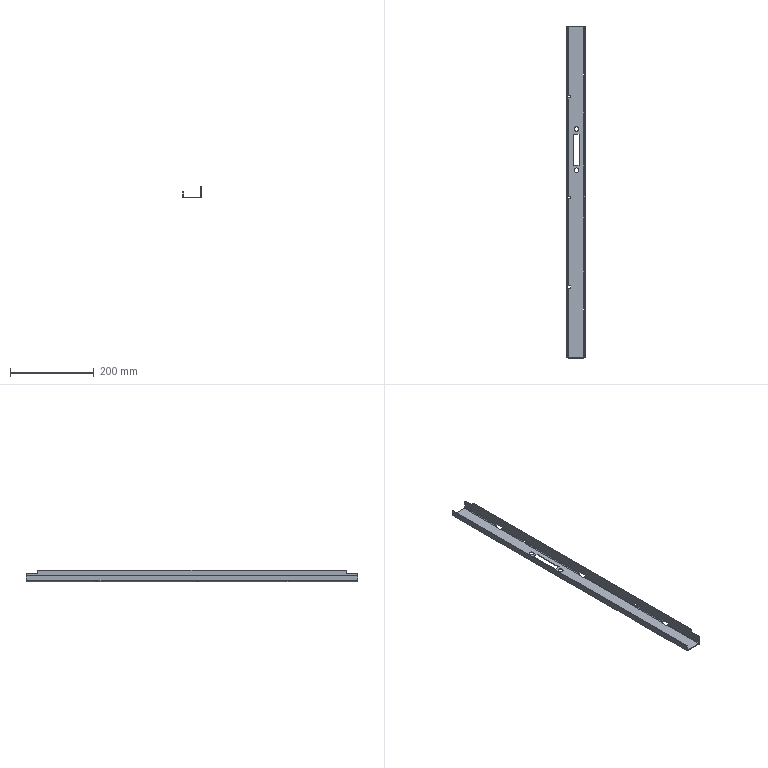Part | STEP file | Middle door gasket strip vertical (door lock) modified | 1 solid | 136 faces | box 44.5 x 791 x 28.5 mm | volume 124119 mm3 | plane 104 | cylinder 32 | commonest cylinder face diameters 3 x14 7 x14 11 x4